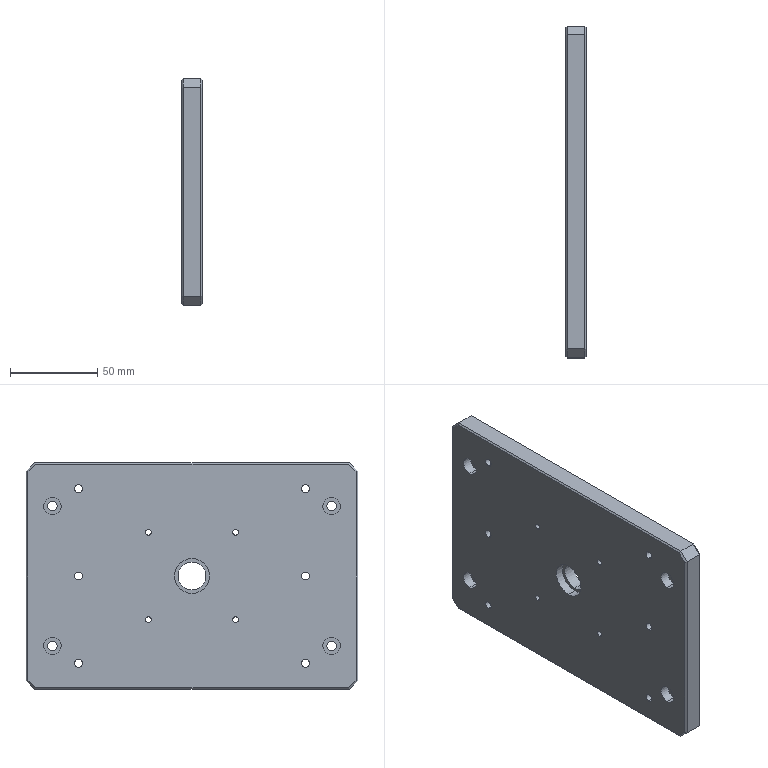Part | STEP file | BPSP-03-013 Test Station Lift Plate_Default | 1 solid | 105 faces | box 12 x 190 x 130 mm | volume 287114 mm3 | cylinder 60 | plane 37 | cone 8 | commonest cylinder face diameters 3.3 x16 4.5 x12 7.5 x12 5.5 x8 10 x8 16 x2